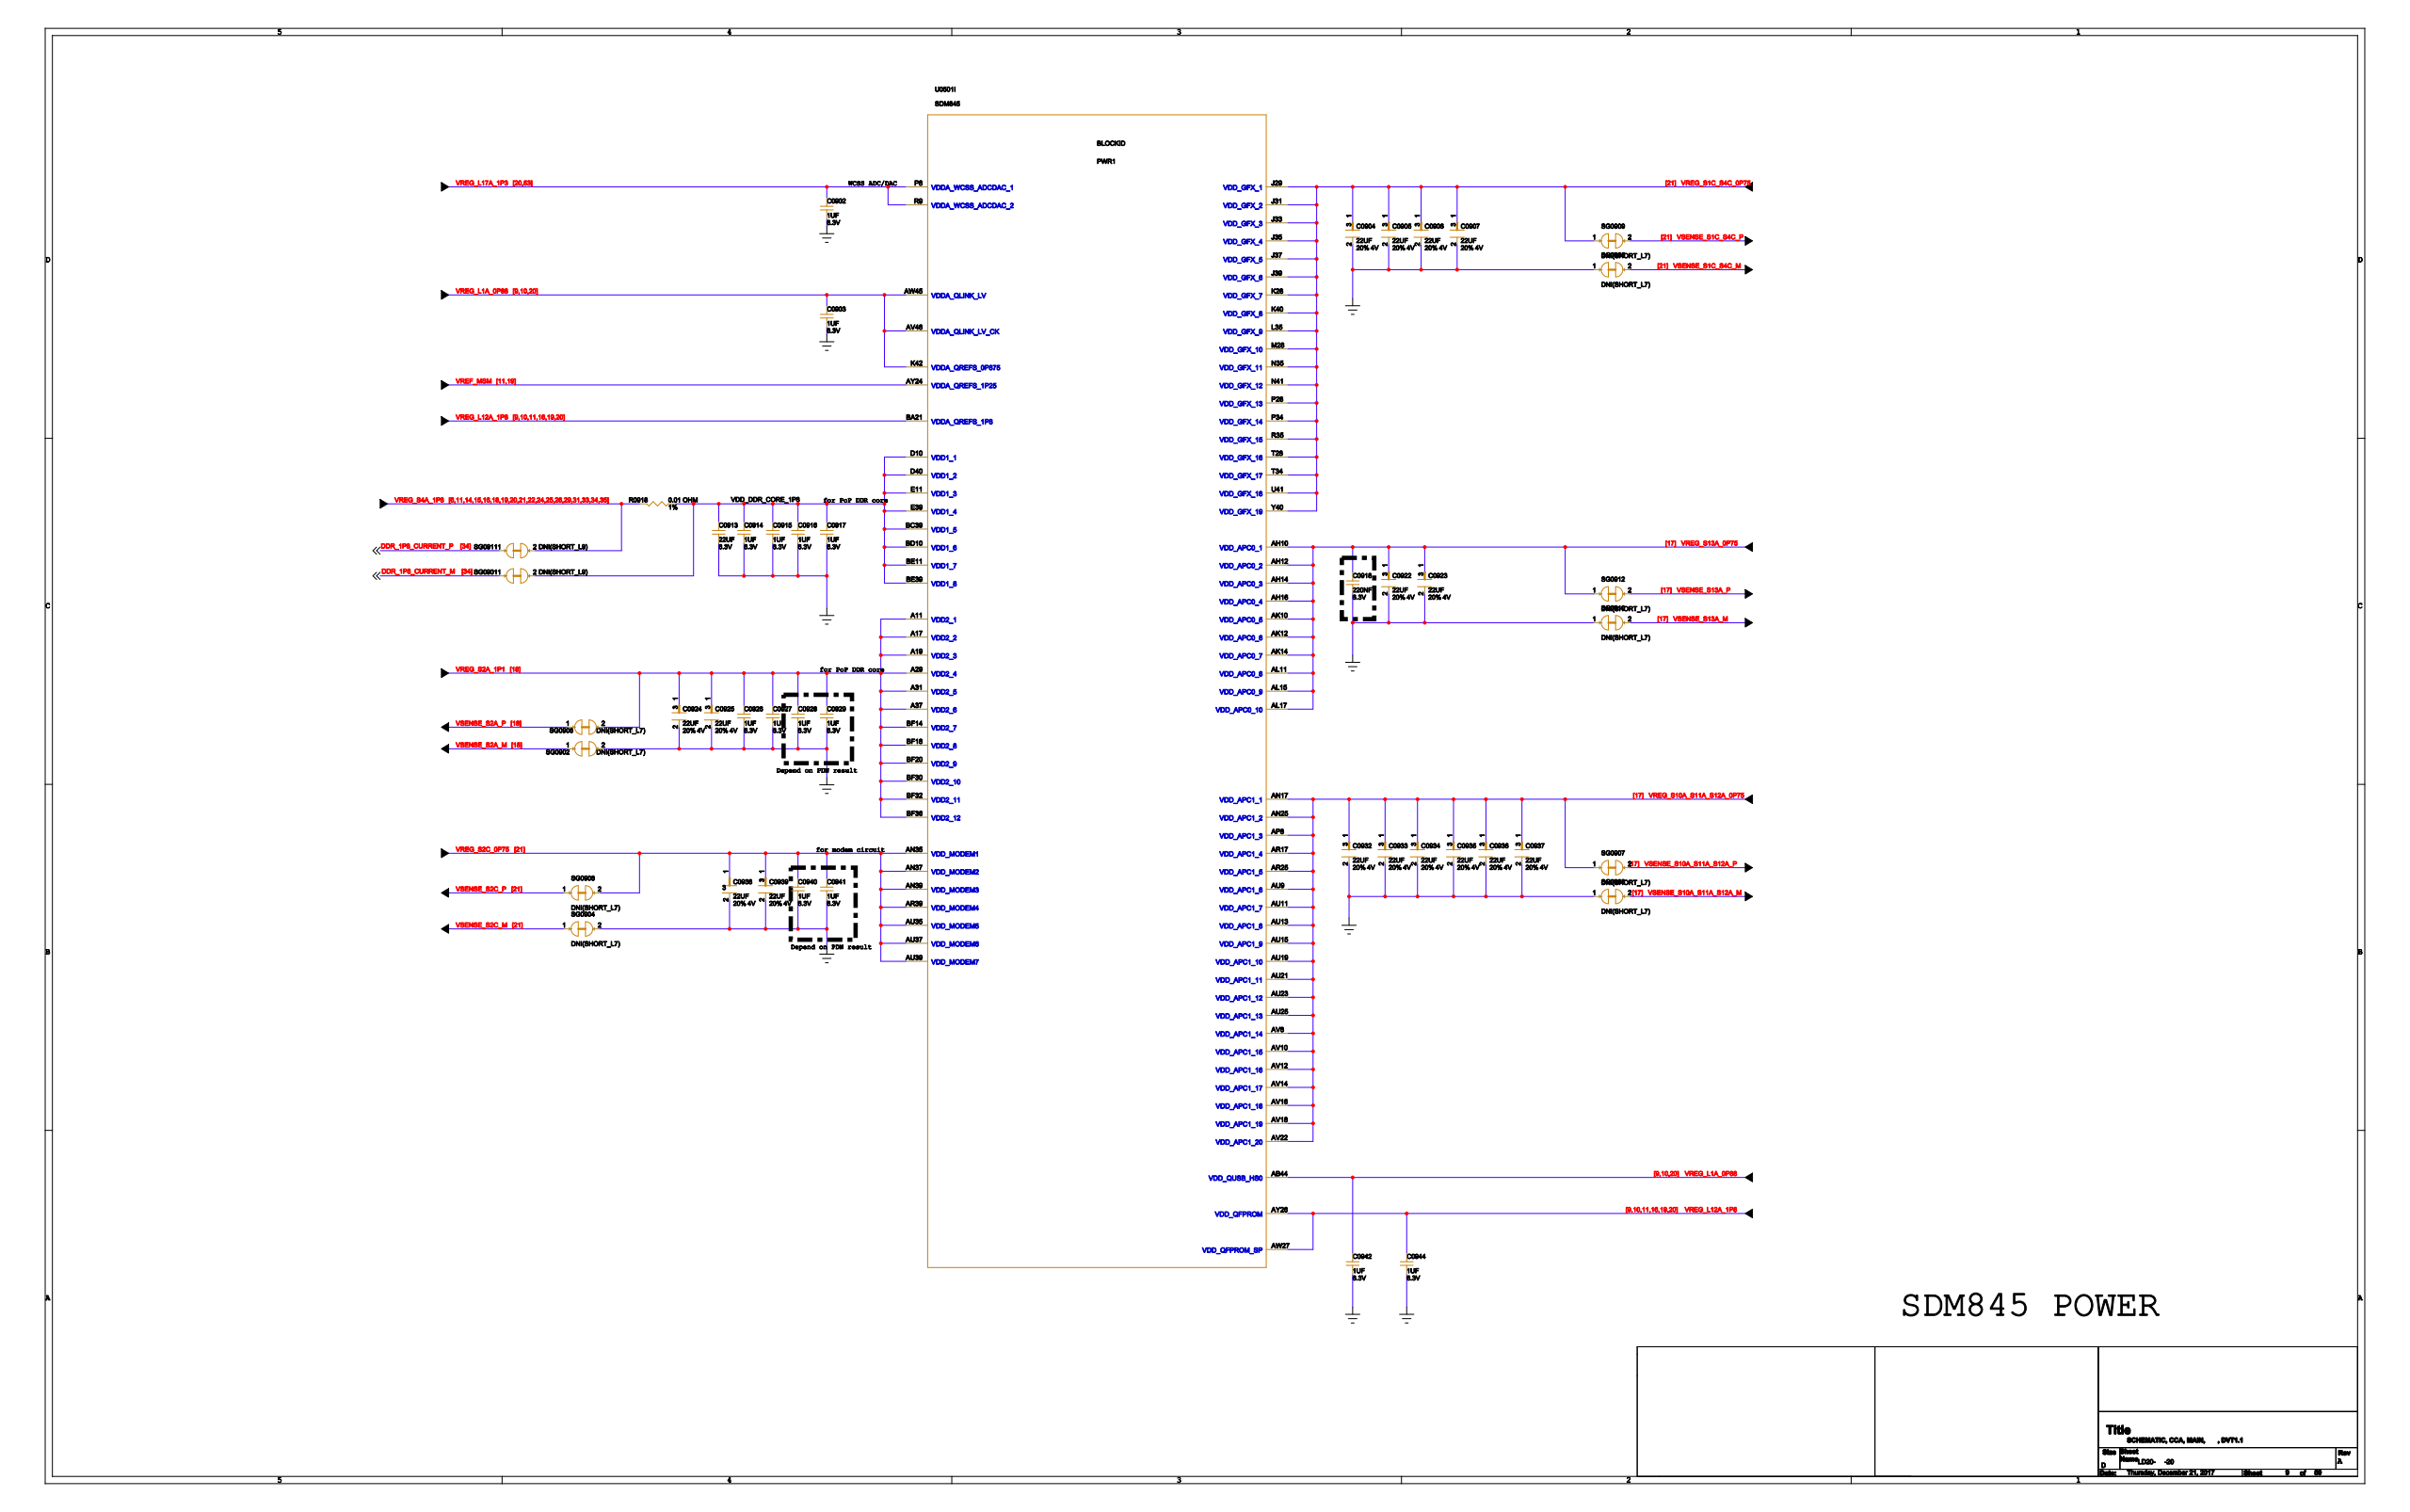Circuit board | Cadence Allegro | 1520 parts | 1149 nets | one sheet of the schematic
Parts on this sheet (reference | value | footprint):
C0902 | 1UF | 2P0201R
C0903 | 1UF | 2P0201R
C0904 | 22UF | 3PSM49X37N
C0905 | 22UF | 3PSM49X37N
C0906 | 22UF | 3PSM49X37N
C0907 | 22UF | 3PSM49X37N
C0913 | 22UF | 2P0603R
C0914 | 1UF | 2P0201R
C0915 | 1UF | 2P0201R
C0916 | 1UF | 2P0201R
C0917 | 1UF | 2P0201R
C0918 | 220NF | 2P0201R
C0922 | 22UF | 3PSM49X37N
C0923 | 22UF | 3PSM49X37N
C0924 | 22UF | 3PSM49X37N
C0925 | 22UF | 3PSM49X37N
C0926 | 1UF | 2P0201R
C0927 | 1UF | 2P0201R
C0928 | 1UF | 2P0201R
C0929 | 1UF | 2P0201R
C0932 | 22UF | 3PSM49X37N
C0933 | 22UF | 3PSM49X37N
C0934 | 22UF | 3PSM49X37N
C0935 | 22UF | 3PSM49X37N
C0936 | 22UF | 3PSM49X37N
C0937 | 22UF | 3PSM49X37N
C0938 | 22UF | 3PSM49X37N
C0939 | 22UF | 3PSM49X37N
C0940 | 1UF | 2P0201R
C0941 | 1UF | 2P0201R
C0942 | 1UF | 2P0201R
C0944 | 1UF | 2P0201R
R0918 | 0.01 OHM | 2P0603R
SG0902 | DNI(SHORT_L7) | SHORT_L7_2REC08X12
SG0903 | DNI(SHORT_L7) | SHORT_L7_2REC08X12
SG0904 | DNI(SHORT_L7) | SHORT_L7_2REC08X12
SG0905 | DNI(SHORT_L7) | SHORT_L7_2REC08X12
SG0906 | DNI(SHORT_L7) | SHORT_L7_2REC08X12
SG0907 | DNI(SHORT_L7) | SHORT_L7_2REC08X12
SG0908 | DNI(SHORT_L7) | SHORT_L7_2REC08X12
SG0909 | DNI(SHORT_L7) | SHORT_L7_2REC08X12
SG0910 | DNI(SHORT_L7) | SHORT_L7_2REC08X12
SG0912 | DNI(SHORT_L7) | SHORT_L7_2REC08X12
U0501 | SDM845 | 914PGA490X490B138D45
Nets of these parts (net: part-pin ...):
GND: C0902-2 C0903-2 C0904-2 C0905-2 C0906-2 C0907-2 C0913-2 C0914-2 C0915-2 C0916-2 C0917-2 C0918-2 C0922-2 C0923-2 C0924-2 C0925-2 C0926-2 C0927-2 C0928-2 C0929-2 C0932-2 C0933-2 C0934-2 C0935-2 C0936-2 C0937-2 C0938-2 C0939-2 C0940-2 C0941-2 C0942-2 C0944-2 SG0902-2 SG0903-1 SG0904-2 SG0905-1 SG0910-1
VREG_S4A_1P8: R0918-1
VDD_DDR_CORE_1P8: C0913-1 C0914-1 C0915-1 C0916-1 C0917-1 R0918-2 U0501-BC39 U0501-BD10 U0501-BE11 U0501-BE39 U0501-D10 U0501-D40 U0501-E11 U0501-E39
VREG_S13A_0P75: C0918-1 C0922-1 C0922-3 C0923-1 C0923-3 SG0912-1 U0501-AH10 U0501-AH12 U0501-AH14 U0501-AH16 U0501-AK10 U0501-AK12 U0501-AK14 U0501-AL11 U0501-AL15 U0501-AL17
VREG_S2A_1P1: C0924-1 C0924-3 C0925-1 C0925-3 C0926-1 C0927-1 C0928-1 C0929-1 SG0906-2 U0501-A11 U0501-A17 U0501-A19 U0501-A29 U0501-A31 U0501-A37 U0501-BF14 U0501-BF18 U0501-BF20 U0501-BF30 U0501-BF32 U0501-BF36
VREG_S2C_0P75: C0938-1 C0938-3 C0939-1 C0939-3 C0940-1 C0941-1 SG0908-2 U0501-AN35 U0501-AN37 U0501-AN39 U0501-AR39 U0501-AU35 U0501-AU37 U0501-AU39
VREG_L12A_1P8: C0944-1 U0501-AW27 U0501-AY26 U0501-BA21
VREF_MSM: U0501-AY24
VREG_L17A_1P3: C0902-1 U0501-P8 U0501-R9
VREG_L1A_0P88: C0903-1 C0942-1 U0501-AB44 U0501-AV46 U0501-AW45 U0501-K42
VREG_S1C_S4C_0P75: C0904-1 C0904-3 C0905-1 C0905-3 C0906-1 C0906-3 C0907-1 C0907-3 SG0909-1 U0501-J29 U0501-J31 U0501-J33 U0501-J35 U0501-J37 U0501-J39 U0501-K28 U0501-K40 U0501-L35 U0501-M28 U0501-N35 U0501-N41 U0501-P28 U0501-P34 U0501-R35 U0501-T28 U0501-T34 U0501-U41 U0501-Y40
VREG_S10A_S11A_S12A_0P75: C0932-1 C0932-3 C0933-1 C0933-3 C0934-1 C0934-3 C0935-1 C0935-3 C0936-1 C0936-3 C0937-1 C0937-3 SG0907-1 U0501-AN17 U0501-AN25 U0501-AP8 U0501-AR17 U0501-AR25 U0501-AU9 U0501-AU11 U0501-AU13 U0501-AU15 U0501-AU19 U0501-AU21 U0501-AU23 U0501-AU25 U0501-AV8 U0501-AV10 U0501-AV12 U0501-AV14 U0501-AV16 U0501-AV18 U0501-AV22
VSENSE_S2A_M: SG0902-1
VSENSE_S10A_S11A_S12A_M: SG0903-2
VSENSE_S2C_M: SG0904-1
VSENSE_S1C_S4C_M: SG0905-2
VSENSE_S2A_P: SG0906-1
VSENSE_S10A_S11A_S12A_P: SG0907-2
VSENSE_S2C_P: SG0908-1
VSENSE_S1C_S4C_P: SG0909-2
VSENSE_S13A_M: SG0910-2
VSENSE_S13A_P: SG0912-2